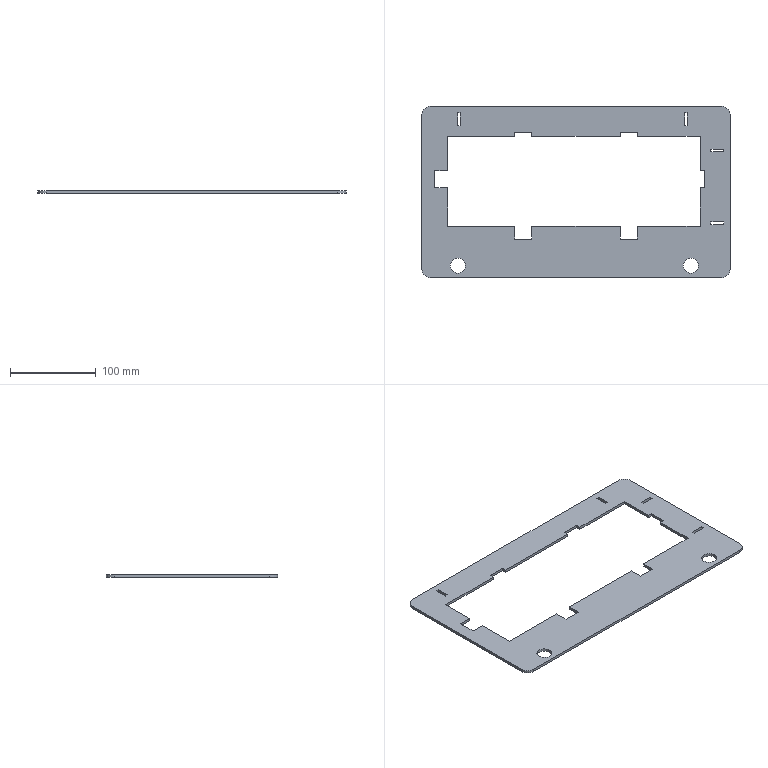Part | SolidWorks | features FlatPattern 1, SMBaseFlange 1, SheetMetal 1 | 1 solid | 58 faces | box 360 x 200 x 3.2 mm | volume 125012 mm3 | plane 50 | cylinder 8 | commonest cylinder face diameters 17.5 x4 20 x4